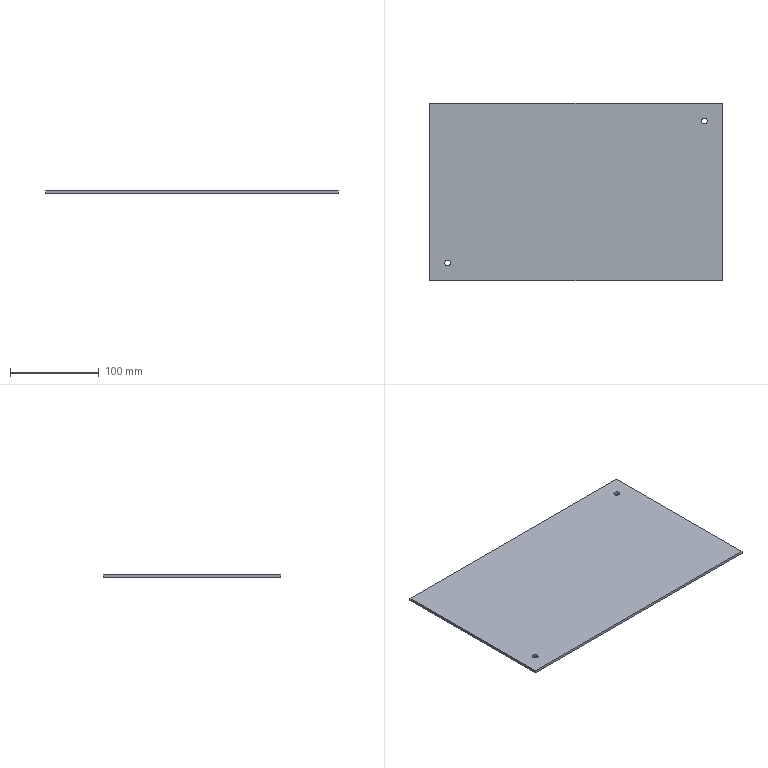Part | SolidWorks | features Extrusion 1, ICE 1 | 1 solid | 10 faces | box 330 x 200 x 3 mm | volume 197807 mm3 | plane 6 | cylinder 4 | commonest cylinder face diameters 6.4 x4
STEP:
#1=CARTESIAN_POINT('',(-148.2,-80.,-1.5));
#2=VERTEX_POINT('',#1);
#3=CARTESIAN_POINT('',(-141.8,-80.,-1.5));
#4=VERTEX_POINT('',#3);
#5=CARTESIAN_POINT('',(-145.,-80.,-1.5));
#6=DIRECTION('',(0.,0.,1.));
#7=DIRECTION('',(1.,0.,0.));
#8=AXIS2_PLACEMENT_3D('',#5,#6,#7);
#9=CIRCLE('',#8,3.2);
#10=EDGE_CURVE('',#2,#4,#9,.T.);
#11=ORIENTED_EDGE('',*,*,#10,.F.);
#12=CARTESIAN_POINT('',(-148.2,-80.,1.5));
#13=VERTEX_POINT('',#12);
#14=CARTESIAN_POINT('',(-148.2,-80.,-11.5));
#15=DIRECTION('',(0.,0.,1.));
#16=VECTOR('',#15,1000.);
#17=LINE('',#14,#16);
#18=EDGE_CURVE('',#2,#13,#17,.T.);
#19=ORIENTED_EDGE('',*,*,#18,.T.);
#20=CARTESIAN_POINT('',(-141.8,-80.,1.5));
#21=VERTEX_POINT('',#20);
#22=CARTESIAN_POINT('',(-145.,-80.,1.5));
#23=DIRECTION('',(0.,0.,1.));
#24=DIRECTION('',(1.,0.,0.));
#25=AXIS2_PLACEMENT_3D('',#22,#23,#24);
#26=CIRCLE('',#25,3.2);
#27=EDGE_CURVE('',#13,#21,#26,.T.);
#28=ORIENTED_EDGE('',*,*,#27,.T.);
#29=CARTESIAN_POINT('',(-141.8,-80.,-11.5));
#30=DIRECTION('',(0.,0.,1.));
#31=VECTOR('',#30,1000.);
#32=LINE('',#29,#31);
#33=EDGE_CURVE('',#4,#21,#32,.T.);
#34=ORIENTED_EDGE('',*,*,#33,.F.);
#35=EDGE_LOOP('',(#11,#19,#28,#34));
#36=FACE_OUTER_BOUND('',#35,.T.);
#37=CARTESIAN_POINT('',(-145.,-80.,-11.5));
#38=DIRECTION('',(0.,0.,1.));
#39=DIRECTION('',(1.,0.,0.));
#40=AXIS2_PLACEMENT_3D('',#37,#38,#39);
#41=CYLINDRICAL_SURFACE('',#40,3.2);
#42=ADVANCED_FACE('',(#36),#41,.F.);
#43=CARTESIAN_POINT('',(141.8,80.,-1.5));
#44=VERTEX_POINT('',#43);
#45=CARTESIAN_POINT('',(148.2,80.,-1.5));
#46=VERTEX_POINT('',#45);
#47=CARTESIAN_POINT('',(145.,80.,-1.5));
#48=DIRECTION('',(0.,0.,1.));
#49=DIRECTION('',(1.,0.,0.));
#50=AXIS2_PLACEMENT_3D('',#47,#48,#49);
#51=CIRCLE('',#50,3.2);
#52=EDGE_CURVE('',#44,#46,#51,.T.);
#53=ORIENTED_EDGE('',*,*,#52,.F.);
#54=CARTESIAN_POINT('',(141.8,80.,1.5));
#55=VERTEX_POINT('',#54);
#56=CARTESIAN_POINT('',(141.8,80.,-11.5));
#57=DIRECTION('',(0.,0.,1.));
#58=VECTOR('',#57,1000.);
#59=LINE('',#56,#58);
#60=EDGE_CURVE('',#44,#55,#59,.T.);
#61=ORIENTED_EDGE('',*,*,#60,.T.);
#62=CARTESIAN_POINT('',(148.2,80.,1.5));
#63=VERTEX_POINT('',#62);
#64=CARTESIAN_POINT('',(145.,80.,1.5));
#65=DIRECTION('',(0.,0.,1.));
#66=DIRECTION('',(1.,0.,0.));
#67=AXIS2_PLACEMENT_3D('',#64,#65,#66);
#68=CIRCLE('',#67,3.2);
#69=EDGE_CURVE('',#55,#63,#68,.T.);
#70=ORIENTED_EDGE('',*,*,#69,.T.);
#71=CARTESIAN_POINT('',(148.2,80.,-11.5));
#72=DIRECTION('',(0.,0.,1.));
#73=VECTOR('',#72,1000.);
#74=LINE('',#71,#73);
#75=EDGE_CURVE('',#46,#63,#74,.T.);
#76=ORIENTED_EDGE('',*,*,#75,.F.);
#77=EDGE_LOOP('',(#53,#61,#70,#76));
#78=FACE_OUTER_BOUND('',#77,.T.);
#79=CARTESIAN_POINT('',(145.,80.,-11.5));
#80=DIRECTION('',(0.,0.,1.));
#81=DIRECTION('',(1.,0.,0.));
#82=AXIS2_PLACEMENT_3D('',#79,#80,#81);
#83=CYLINDRICAL_SURFACE('',#82,3.2);
#84=ADVANCED_FACE('',(#78),#83,.F.);
#85=CARTESIAN_POINT('',(-165.,100.,1.5));
#86=VERTEX_POINT('',#85);
#87=CARTESIAN_POINT('',(-165.,-100.,1.5));
#88=VERTEX_POINT('',#87);
#89=CARTESIAN_POINT('',(-165.,100.,1.5));
#90=DIRECTION('',(0.,-1.,0.));
#91=VECTOR('',#90,1000.);
#92=LINE('',#89,#91);
#93=EDGE_CURVE('',#86,#88,#92,.T.);
#94=ORIENTED_EDGE('',*,*,#93,.F.);
#95=CARTESIAN_POINT('',(-165.,100.,-1.5));
#96=VERTEX_POINT('',#95);
#97=CARTESIAN_POINT('',(-165.,100.,-1.5));
#98=DIRECTION('',(0.,0.,1.));
#99=VECTOR('',#98,1000.);
#100=LINE('',#97,#99);
#101=EDGE_CURVE('',#96,#86,#100,.T.);
#102=ORIENTED_EDGE('',*,*,#101,.F.);
#103=CARTESIAN_POINT('',(-165.,-100.,-1.5));
#104=VERTEX_POINT('',#103);
#105=CARTESIAN_POINT('',(-165.,100.,-1.5));
#106=DIRECTION('',(0.,-1.,0.));
#107=VECTOR('',#106,1000.);
#108=LINE('',#105,#107);
#109=EDGE_CURVE('',#96,#104,#108,.T.);
#110=ORIENTED_EDGE('',*,*,#109,.T.);
#111=CARTESIAN_POINT('',(-165.,-100.,-1.5));
#112=DIRECTION('',(0.,0.,1.));
#113=VECTOR('',#112,1000.);
#114=LINE('',#111,#113);
#115=EDGE_CURVE('',#104,#88,#114,.T.);
#116=ORIENTED_EDGE('',*,*,#115,.T.);
#117=EDGE_LOOP('',(#94,#102,#110,#116));
#118=FACE_OUTER_BOUND('',#117,.T.);
#119=CARTESIAN_POINT('',(-165.,100.,-1.5));
#120=DIRECTION('',(-1.,0.,0.));
#121=DIRECTION('',(0.,0.,1.));
#122=AXIS2_PLACEMENT_3D('',#119,#120,#121);
#123=PLANE('',#122);
#124=ADVANCED_FACE('',(#118),#123,.T.);
#125=CARTESIAN_POINT('',(165.,100.,1.5));
#126=VERTEX_POINT('',#125);
#127=CARTESIAN_POINT('',(165.,100.,1.5));
#128=DIRECTION('',(-1.,0.,0.));
#129=VECTOR('',#128,1000.);
#130=LINE('',#127,#129);
#131=EDGE_CURVE('',#126,#86,#130,.T.);
#132=ORIENTED_EDGE('',*,*,#131,.F.);
#133=CARTESIAN_POINT('',(165.,100.,-1.5));
#134=VERTEX_POINT('',#133);
#135=CARTESIAN_POINT('',(165.,100.,-1.5));
#136=DIRECTION('',(0.,0.,1.));
#137=VECTOR('',#136,1000.);
#138=LINE('',#135,#137);
#139=EDGE_CURVE('',#134,#126,#138,.T.);
#140=ORIENTED_EDGE('',*,*,#139,.F.);
#141=CARTESIAN_POINT('',(165.,100.,-1.5));
#142=DIRECTION('',(-1.,0.,0.));
#143=VECTOR('',#142,1000.);
#144=LINE('',#141,#143);
#145=EDGE_CURVE('',#134,#96,#144,.T.);
#146=ORIENTED_EDGE('',*,*,#145,.T.);
#147=ORIENTED_EDGE('',*,*,#101,.T.);
#148=EDGE_LOOP('',(#132,#140,#146,#147));
#149=FACE_OUTER_BOUND('',#148,.T.);
#150=CARTESIAN_POINT('',(165.,100.,-1.5));
#151=DIRECTION('',(0.,1.,0.));
#152=DIRECTION('',(0.,0.,1.));
#153=AXIS2_PLACEMENT_3D('',#150,#151,#152);
#154=PLANE('',#153);
#155=ADVANCED_FACE('',(#149),#154,.T.);
#156=CARTESIAN_POINT('',(165.,-100.,1.5));
#157=VERTEX_POINT('',#156);
#158=CARTESIAN_POINT('',(165.,-100.,1.5));
#159=DIRECTION('',(0.,1.,0.));
#160=VECTOR('',#159,1000.);
#161=LINE('',#158,#160);
#162=EDGE_CURVE('',#157,#126,#161,.T.);
#163=ORIENTED_EDGE('',*,*,#162,.F.);
#164=CARTESIAN_POINT('',(165.,-100.,-1.5));
#165=VERTEX_POINT('',#164);
#166=CARTESIAN_POINT('',(165.,-100.,-1.5));
#167=DIRECTION('',(0.,0.,1.));
#168=VECTOR('',#167,1000.);
#169=LINE('',#166,#168);
#170=EDGE_CURVE('',#165,#157,#169,.T.);
#171=ORIENTED_EDGE('',*,*,#170,.F.);
#172=CARTESIAN_POINT('',(165.,-100.,-1.5));
#173=DIRECTION('',(0.,1.,0.));
#174=VECTOR('',#173,1000.);
#175=LINE('',#172,#174);
#176=EDGE_CURVE('',#165,#134,#175,.T.);
#177=ORIENTED_EDGE('',*,*,#176,.T.);
#178=ORIENTED_EDGE('',*,*,#139,.T.);
#179=EDGE_LOOP('',(#163,#171,#177,#178));
#180=FACE_OUTER_BOUND('',#179,.T.);
#181=CARTESIAN_POINT('',(165.,-100.,-1.5));
#182=DIRECTION('',(1.,0.,0.));
#183=DIRECTION('',(0.,0.,-1.));
#184=AXIS2_PLACEMENT_3D('',#181,#182,#183);
#185=PLANE('',#184);
#186=ADVANCED_FACE('',(#180),#185,.T.);
#187=CARTESIAN_POINT('',(-165.,-100.,1.5));
#188=DIRECTION('',(1.,0.,0.));
#189=VECTOR('',#188,1000.);
#190=LINE('',#187,#189);
#191=EDGE_CURVE('',#88,#157,#190,.T.);
#192=ORIENTED_EDGE('',*,*,#191,.F.);
#193=ORIENTED_EDGE('',*,*,#115,.F.);
#194=CARTESIAN_POINT('',(-165.,-100.,-1.5));
#195=DIRECTION('',(1.,0.,0.));
#196=VECTOR('',#195,1000.);
#197=LINE('',#194,#196);
#198=EDGE_CURVE('',#104,#165,#197,.T.);
#199=ORIENTED_EDGE('',*,*,#198,.T.);
#200=ORIENTED_EDGE('',*,*,#170,.T.);
#201=EDGE_LOOP('',(#192,#193,#199,#200));
#202=FACE_OUTER_BOUND('',#201,.T.);
#203=CARTESIAN_POINT('',(-165.,-100.,-1.5));
#204=DIRECTION('',(0.,-1.,0.));
#205=DIRECTION('',(0.,0.,-1.));
#206=AXIS2_PLACEMENT_3D('',#203,#204,#205);
#207=PLANE('',#206);
#208=ADVANCED_FACE('',(#202),#207,.T.);
#209=CARTESIAN_POINT('',(-145.,-80.,-1.5));
#210=DIRECTION('',(0.,0.,1.));
#211=DIRECTION('',(1.,0.,0.));
#212=AXIS2_PLACEMENT_3D('',#209,#210,#211);
#213=CIRCLE('',#212,3.2);
#214=EDGE_CURVE('',#4,#2,#213,.T.);
#215=ORIENTED_EDGE('',*,*,#214,.T.);
#216=ORIENTED_EDGE('',*,*,#10,.T.);
#217=EDGE_LOOP('',(#215,#216));
#218=FACE_BOUND('',#217,.T.);
#219=CARTESIAN_POINT('',(145.,80.,-1.5));
#220=DIRECTION('',(0.,0.,1.));
#221=DIRECTION('',(1.,0.,0.));
#222=AXIS2_PLACEMENT_3D('',#219,#220,#221);
#223=CIRCLE('',#222,3.2);
#224=EDGE_CURVE('',#46,#44,#223,.T.);
#225=ORIENTED_EDGE('',*,*,#224,.T.);
#226=ORIENTED_EDGE('',*,*,#52,.T.);
#227=EDGE_LOOP('',(#225,#226));
#228=FACE_BOUND('',#227,.T.);
#229=ORIENTED_EDGE('',*,*,#109,.F.);
#230=ORIENTED_EDGE('',*,*,#145,.F.);
#231=ORIENTED_EDGE('',*,*,#176,.F.);
#232=ORIENTED_EDGE('',*,*,#198,.F.);
#233=EDGE_LOOP('',(#229,#230,#231,#232));
#234=FACE_OUTER_BOUND('',#233,.T.);
#235=CARTESIAN_POINT('',(0.,0.,-1.5));
#236=DIRECTION('',(0.,0.,1.));
#237=DIRECTION('',(1.,0.,0.));
#238=AXIS2_PLACEMENT_3D('',#235,#236,#237);
#239=PLANE('',#238);
#240=ADVANCED_FACE('',(#218,#228,#234),#239,.F.);
#241=CARTESIAN_POINT('',(-145.,-80.,1.5));
#242=DIRECTION('',(0.,0.,1.));
#243=DIRECTION('',(1.,0.,0.));
#244=AXIS2_PLACEMENT_3D('',#241,#242,#243);
#245=CIRCLE('',#244,3.2);
#246=EDGE_CURVE('',#21,#13,#245,.T.);
#247=ORIENTED_EDGE('',*,*,#246,.F.);
#248=ORIENTED_EDGE('',*,*,#27,.F.);
#249=EDGE_LOOP('',(#247,#248));
#250=FACE_BOUND('',#249,.T.);
#251=CARTESIAN_POINT('',(145.,80.,1.5));
#252=DIRECTION('',(0.,0.,1.));
#253=DIRECTION('',(1.,0.,0.));
#254=AXIS2_PLACEMENT_3D('',#251,#252,#253);
#255=CIRCLE('',#254,3.2);
#256=EDGE_CURVE('',#63,#55,#255,.T.);
#257=ORIENTED_EDGE('',*,*,#256,.F.);
#258=ORIENTED_EDGE('',*,*,#69,.F.);
#259=EDGE_LOOP('',(#257,#258));
#260=FACE_BOUND('',#259,.T.);
#261=ORIENTED_EDGE('',*,*,#93,.T.);
#262=ORIENTED_EDGE('',*,*,#191,.T.);
#263=ORIENTED_EDGE('',*,*,#162,.T.);
#264=ORIENTED_EDGE('',*,*,#131,.T.);
#265=EDGE_LOOP('',(#261,#262,#263,#264));
#266=FACE_OUTER_BOUND('',#265,.T.);
#267=CARTESIAN_POINT('',(0.,0.,1.5));
#268=DIRECTION('',(0.,0.,1.));
#269=DIRECTION('',(1.,0.,0.));
#270=AXIS2_PLACEMENT_3D('',#267,#268,#269);
#271=PLANE('',#270);
#272=ADVANCED_FACE('',(#250,#260,#266),#271,.T.);
#273=ORIENTED_EDGE('',*,*,#60,.F.);
#274=ORIENTED_EDGE('',*,*,#224,.F.);
#275=ORIENTED_EDGE('',*,*,#75,.T.);
#276=ORIENTED_EDGE('',*,*,#256,.T.);
#277=EDGE_LOOP('',(#273,#274,#275,#276));
#278=FACE_OUTER_BOUND('',#277,.T.);
#279=CARTESIAN_POINT('',(145.,80.,-11.5));
#280=DIRECTION('',(0.,0.,1.));
#281=DIRECTION('',(1.,0.,0.));
#282=AXIS2_PLACEMENT_3D('',#279,#280,#281);
#283=CYLINDRICAL_SURFACE('',#282,3.2);
#284=ADVANCED_FACE('',(#278),#283,.F.);
#285=ORIENTED_EDGE('',*,*,#18,.F.);
#286=ORIENTED_EDGE('',*,*,#214,.F.);
#287=ORIENTED_EDGE('',*,*,#33,.T.);
#288=ORIENTED_EDGE('',*,*,#246,.T.);
#289=EDGE_LOOP('',(#285,#286,#287,#288));
#290=FACE_OUTER_BOUND('',#289,.T.);
#291=CARTESIAN_POINT('',(-145.,-80.,-11.5));
#292=DIRECTION('',(0.,0.,1.));
#293=DIRECTION('',(1.,0.,0.));
#294=AXIS2_PLACEMENT_3D('',#291,#292,#293);
#295=CYLINDRICAL_SURFACE('',#294,3.2);
#296=ADVANCED_FACE('',(#290),#295,.F.);
#297=CLOSED_SHELL('',(#42,#84,#124,#155,#186,#208,#240,#272,#284,#296));
#298=MANIFOLD_SOLID_BREP('',#297);
#299=CARTESIAN_POINT('',(0.,0.,0.));
#300=DIRECTION('',(0.,0.,1.));
#301=DIRECTION('',(1.,0.,0.));
#302=AXIS2_PLACEMENT_3D('',#299,#300,#301);
#303=(LENGTH_UNIT()NAMED_UNIT(*)SI_UNIT(.MILLI.,.METRE.));
#304=UNCERTAINTY_MEASURE_WITH_UNIT(LENGTH_MEASURE(0.00001),#303,'','');
#305=(NAMED_UNIT(*)PLANE_ANGLE_UNIT()SI_UNIT($,.RADIAN.));
#306=(NAMED_UNIT(*)SI_UNIT($,.STERADIAN.)SOLID_ANGLE_UNIT());
#307=(GEOMETRIC_REPRESENTATION_CONTEXT(3)GLOBAL_UNCERTAINTY_ASSIGNED_CONTEXT((#304))GLOBAL_UNIT_ASSIGNED_CONTEXT((#303,#305,#306))REPRESENTATION_CONTEXT('',''));
#308=ADVANCED_BREP_SHAPE_REPRESENTATION('',(#298,#302),#307);